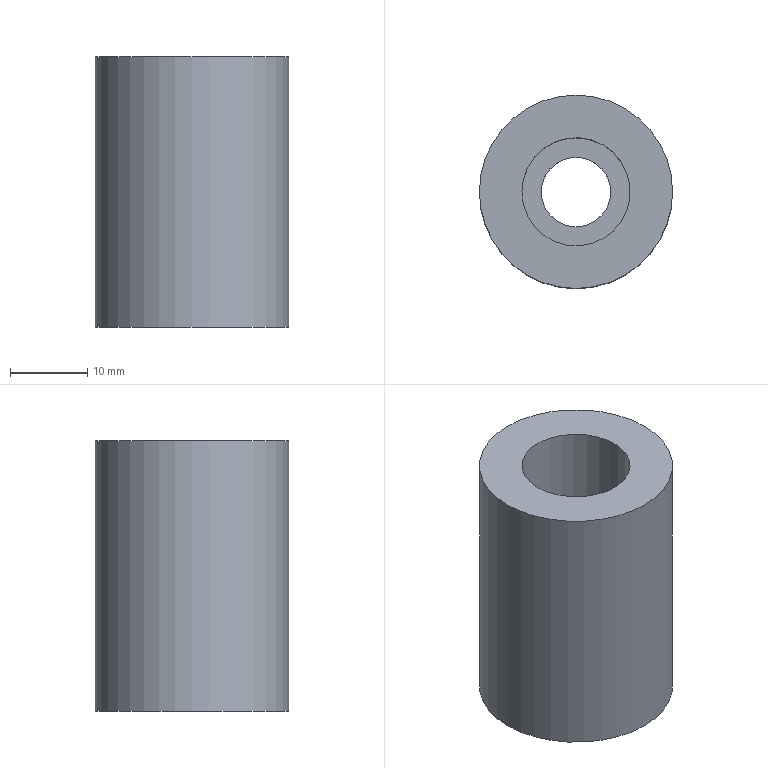Part | NX | features solid 2 | 1 solid | 6 faces | box 25 x 25 x 35 mm | volume 13148 mm3 | plane 3 | cylinder 3 | commonest cylinder face diameters 9 x1 14 x1 25 x1
STEP:
#1=CARTESIAN_POINT('',(-4.5,-245.,5.));
#2=VERTEX_POINT('',#1);
#3=CARTESIAN_POINT('',(0.,-245.,5.));
#4=DIRECTION('',(0.,0.,-1.));
#5=DIRECTION('',(-1.,0.,0.));
#6=AXIS2_PLACEMENT_3D('',#3,#4,#5);
#7=CIRCLE('',#6,4.5);
#8=EDGE_CURVE('',#2,#2,#7,.T.);
#9=ORIENTED_EDGE('',*,*,#8,.F.);
#10=EDGE_LOOP('',(#9));
#11=FACE_BOUND('',#10,.T.);
#12=CARTESIAN_POINT('',(-12.5,-245.,5.));
#13=VERTEX_POINT('',#12);
#14=CARTESIAN_POINT('',(0.,-245.,5.));
#15=DIRECTION('',(0.,0.,-1.));
#16=DIRECTION('',(-1.,0.,0.));
#17=AXIS2_PLACEMENT_3D('',#14,#15,#16);
#18=CIRCLE('',#17,12.5);
#19=EDGE_CURVE('',#13,#13,#18,.F.);
#20=ORIENTED_EDGE('',*,*,#19,.F.);
#21=EDGE_LOOP('',(#20));
#22=FACE_BOUND('',#21,.T.);
#23=CARTESIAN_POINT('',(0.,-245.,5.));
#24=DIRECTION('',(0.,0.,-1.));
#25=DIRECTION('',(-1.,0.,0.));
#26=AXIS2_PLACEMENT_3D('',#23,#24,#25);
#27=PLANE('',#26);
#28=ADVANCED_FACE('',(#11,#22),#27,.T.);
#29=CARTESIAN_POINT('',(-7.,-245.,40.));
#30=VERTEX_POINT('',#29);
#31=CARTESIAN_POINT('',(0.,-245.,40.));
#32=DIRECTION('',(0.,0.,-1.));
#33=DIRECTION('',(-1.,0.,0.));
#34=AXIS2_PLACEMENT_3D('',#31,#32,#33);
#35=CIRCLE('',#34,7.);
#36=EDGE_CURVE('',#30,#30,#35,.T.);
#37=ORIENTED_EDGE('',*,*,#36,.T.);
#38=EDGE_LOOP('',(#37));
#39=FACE_BOUND('',#38,.T.);
#40=CARTESIAN_POINT('',(-12.5,-245.,40.));
#41=VERTEX_POINT('',#40);
#42=CARTESIAN_POINT('',(0.,-245.,40.));
#43=DIRECTION('',(0.,0.,-1.));
#44=DIRECTION('',(-1.,0.,0.));
#45=AXIS2_PLACEMENT_3D('',#42,#43,#44);
#46=CIRCLE('',#45,12.5);
#47=EDGE_CURVE('',#41,#41,#46,.F.);
#48=ORIENTED_EDGE('',*,*,#47,.T.);
#49=EDGE_LOOP('',(#48));
#50=FACE_BOUND('',#49,.T.);
#51=CARTESIAN_POINT('',(0.,-242.5,40.));
#52=DIRECTION('',(0.,0.,-1.));
#53=DIRECTION('',(0.,1.,0.));
#54=AXIS2_PLACEMENT_3D('',#51,#52,#53);
#55=PLANE('',#54);
#56=ADVANCED_FACE('',(#39,#50),#55,.F.);
#57=ORIENTED_EDGE('',*,*,#47,.F.);
#58=EDGE_LOOP('',(#57));
#59=FACE_BOUND('',#58,.T.);
#60=ORIENTED_EDGE('',*,*,#19,.T.);
#61=EDGE_LOOP('',(#60));
#62=FACE_BOUND('',#61,.T.);
#63=CARTESIAN_POINT('',(0.,-245.,-37.));
#64=DIRECTION('',(0.,0.,1.));
#65=DIRECTION('',(0.,1.,0.));
#66=AXIS2_PLACEMENT_3D('',#63,#64,#65);
#67=CYLINDRICAL_SURFACE('',#66,12.5);
#68=ADVANCED_FACE('',(#59,#62),#67,.T.);
#69=ORIENTED_EDGE('',*,*,#8,.T.);
#70=EDGE_LOOP('',(#69));
#71=FACE_BOUND('',#70,.T.);
#72=CARTESIAN_POINT('',(-4.5,-245.,20.));
#73=VERTEX_POINT('',#72);
#74=CARTESIAN_POINT('',(0.,-245.,20.));
#75=DIRECTION('',(0.,0.,-1.));
#76=DIRECTION('',(-1.,0.,0.));
#77=AXIS2_PLACEMENT_3D('',#74,#75,#76);
#78=CIRCLE('',#77,4.5);
#79=EDGE_CURVE('',#73,#73,#78,.T.);
#80=ORIENTED_EDGE('',*,*,#79,.F.);
#81=EDGE_LOOP('',(#80));
#82=FACE_BOUND('',#81,.T.);
#83=CARTESIAN_POINT('',(0.,-245.,-10.));
#84=DIRECTION('',(0.,0.,-1.));
#85=DIRECTION('',(-1.,0.,0.));
#86=AXIS2_PLACEMENT_3D('',#83,#84,#85);
#87=CYLINDRICAL_SURFACE('',#86,4.5);
#88=ADVANCED_FACE('',(#71,#82),#87,.F.);
#89=ORIENTED_EDGE('',*,*,#79,.T.);
#90=EDGE_LOOP('',(#89));
#91=FACE_BOUND('',#90,.T.);
#92=CARTESIAN_POINT('',(-7.,-245.,20.));
#93=VERTEX_POINT('',#92);
#94=CARTESIAN_POINT('',(0.,-245.,20.));
#95=DIRECTION('',(0.,0.,-1.));
#96=DIRECTION('',(-1.,0.,0.));
#97=AXIS2_PLACEMENT_3D('',#94,#95,#96);
#98=CIRCLE('',#97,7.);
#99=EDGE_CURVE('',#93,#93,#98,.T.);
#100=ORIENTED_EDGE('',*,*,#99,.F.);
#101=EDGE_LOOP('',(#100));
#102=FACE_BOUND('',#101,.T.);
#103=CARTESIAN_POINT('',(0.,-245.,20.));
#104=DIRECTION('',(0.,0.,-1.));
#105=DIRECTION('',(-1.,0.,0.));
#106=AXIS2_PLACEMENT_3D('',#103,#104,#105);
#107=PLANE('',#106);
#108=ADVANCED_FACE('',(#91,#102),#107,.F.);
#109=ORIENTED_EDGE('',*,*,#99,.T.);
#110=EDGE_LOOP('',(#109));
#111=FACE_BOUND('',#110,.T.);
#112=ORIENTED_EDGE('',*,*,#36,.F.);
#113=EDGE_LOOP('',(#112));
#114=FACE_BOUND('',#113,.T.);
#115=CARTESIAN_POINT('',(0.,-245.,40.));
#116=DIRECTION('',(0.,0.,-1.));
#117=DIRECTION('',(-1.,0.,0.));
#118=AXIS2_PLACEMENT_3D('',#115,#116,#117);
#119=CYLINDRICAL_SURFACE('',#118,7.);
#120=ADVANCED_FACE('',(#111,#114),#119,.F.);
#121=CLOSED_SHELL('',(#28,#56,#68,#88,#108,#120));
#122=MANIFOLD_SOLID_BREP('',#121);
#123=(LENGTH_UNIT()NAMED_UNIT(*)SI_UNIT(.MILLI.,.METRE.));
#124=UNCERTAINTY_MEASURE_WITH_UNIT(LENGTH_MEASURE(0.00001),#123,'','');
#125=(NAMED_UNIT(*)PLANE_ANGLE_UNIT()SI_UNIT($,.RADIAN.));
#126=(NAMED_UNIT(*)SI_UNIT($,.STERADIAN.)SOLID_ANGLE_UNIT());
#127=(GEOMETRIC_REPRESENTATION_CONTEXT(3)GLOBAL_UNCERTAINTY_ASSIGNED_CONTEXT((#124))GLOBAL_UNIT_ASSIGNED_CONTEXT((#123,#125,#126))REPRESENTATION_CONTEXT('',''));
#128=ADVANCED_BREP_SHAPE_REPRESENTATION('',(#122),#127);